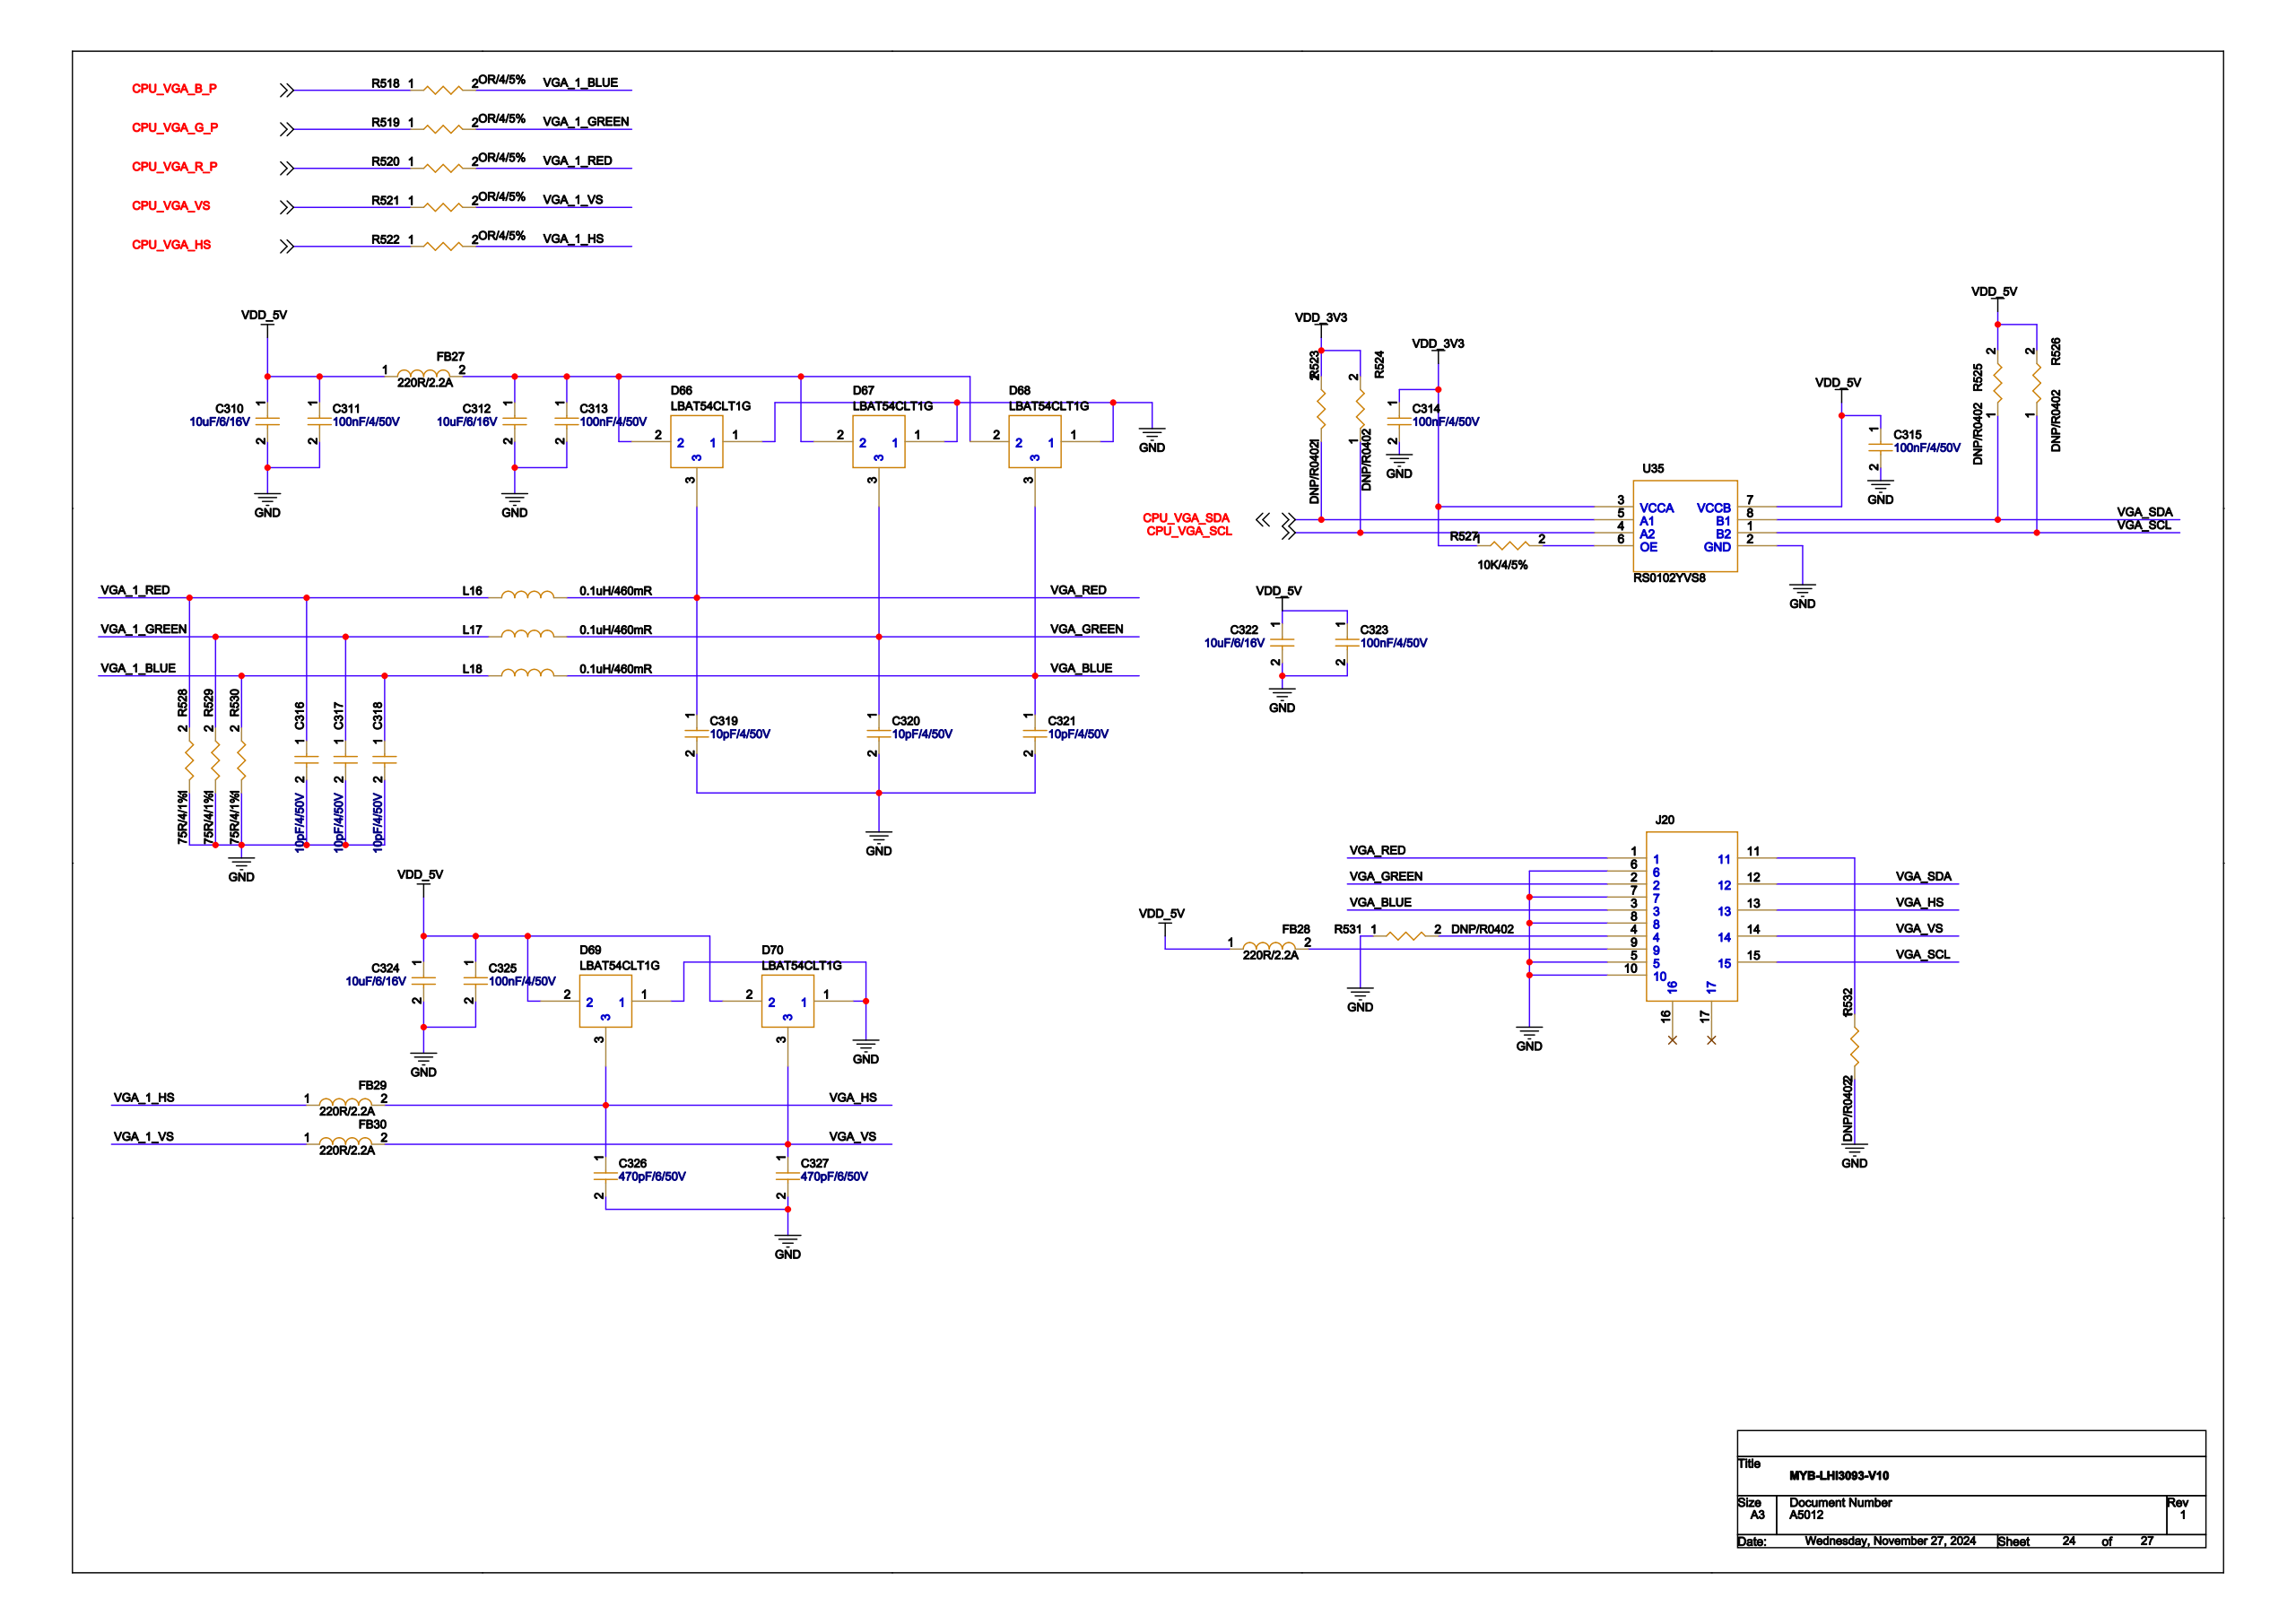Circuit board | Cadence Allegro | 1159 parts | 708 nets | one sheet of the schematic
Parts on this sheet (reference | value | footprint):
C310 | 10uF/6/16V | C0603
C311 | 100nF/4/50V | C0402
C312 | 10uF/6/16V | C0603
C313 | 100nF/4/50V | C0402
C314 | 100nF/4/50V | C0402
C315 | 100nF/4/50V | C0402
C316 | 10pF/4/50V | C0402
C317 | 10pF/4/50V | C0402
C318 | 10pF/4/50V | C0402
C319 | 10pF/4/50V | C0402
C320 | 10pF/4/50V | C0402
C321 | 10pF/4/50V | C0402
C322 | 10uF/6/16V | C0402
C323 | 100nF/4/50V | C0402
C324 | 10uF/6/16V | C0603
C325 | 100nF/4/50V | C0402
C326 | 470pF/6/50V | C0603
C327 | 470pF/6/50V | C0603
D66 | LBAT54CLT1G | SOT-23
D67 | LBAT54CLT1G | SOT-23
D68 | LBAT54CLT1G | SOT-23
D69 | LBAT54CLT1G | SOT-23
D70 | LBAT54CLT1G | SOT-23
FB27 | 220R/2.2A | FB0603
FB28 | 220R/2.2A | FB0603
FB29 | 220R/2.2A | FB0603
FB30 | 220R/2.2A | FB0603
J20 | DB17 | HDR-15P-3_08
L16 | 0.1uH/460mR | L0805
L17 | 0.1uH/460mR | L0805
L18 | 0.1uH/460mR | L0805
R518 | OR/4/5% | R0402
R519 | OR/4/5% | R0402
R520 | OR/4/5% | R0402
R521 | OR/4/5% | R0402
R522 | OR/4/5% | R0402
R523 | DNP/R0402 | R0402
R524 | DNP/R0402 | R0402
R525 | DNP/R0402 | R0402
R526 | DNP/R0402 | R0402
R527 | 10K/4/5% | R0402
R528 | 75R/4/1% | R0402
R529 | 75R/4/1% | R0402
R530 | 75R/4/1% | R0402
R531 | DNP/R0402 | R0402
R532 | DNP/R0402 | R0402
U35 | RS0102YVS8 | VSSOP8
Nets of these parts (net: part-pin ...):
GND: C310-2 C311-2 C312-2 C313-2 C314-2 C315-2 C316-2 C317-2 C318-2 C319-2 C320-2 C321-2 C322-2 C323-2 C324-2 C325-2 C326-2 C327-2 D66-1 D67-1 D68-1 D69-1 D70-1 J20-5 J20-6 J20-7 J20-8 J20-10 R528-1 R529-1 R530-1 R531-1 R532-2 U35-2
VDD_5V: C310-1 C311-1 C315-1 C322-1 C323-1 C324-1 C325-1 D69-2 D70-2 FB27-1 FB28-1 R525-2 R526-2 U35-7
VDD_3V3: C314-1 R523-2 R524-2 R527-1 U35-3
N15099762: C312-1 C313-1 D66-2 D67-2 D68-2 FB27-2
VGA_1_RED: C316-1 L16-1 R520-2 R528-2
VGA_1_GREEN: C317-1 L17-1 R519-2 R529-2
VGA_1_BLUE: C318-1 L18-1 R518-2 R530-2
VGA_RED: C319-1 D66-3 J20-1 L16-2
VGA_GREEN: C320-1 D67-3 J20-2 L17-2
VGA_BLUE: C321-1 D68-3 J20-3 L18-2
VGA_HS: C326-1 D69-3 FB29-2 J20-13
VGA_VS: C327-1 D70-3 FB30-2 J20-14
N15106167: FB28-2 J20-9
VGA_1_HS: FB29-1 R522-2
VGA_1_VS: FB30-1 R521-2
N15105688: J20-11 R532-1
VGA_SDA: J20-12 R525-1 U35-8
VGA_SCL: J20-15 R526-1 U35-1
N15106269: J20-4 R531-2
N15104012: R527-2 U35-6
CPU_VGA_SDA: R523-1 U35-5
CPU_VGA_SCL: R524-1 U35-4
CPU_VGA_B_P: R518-1
CPU_VGA_G_P: R519-1
CPU_VGA_R_P: R520-1
CPU_VGA_VS: R521-1
CPU_VGA_HS: R522-1